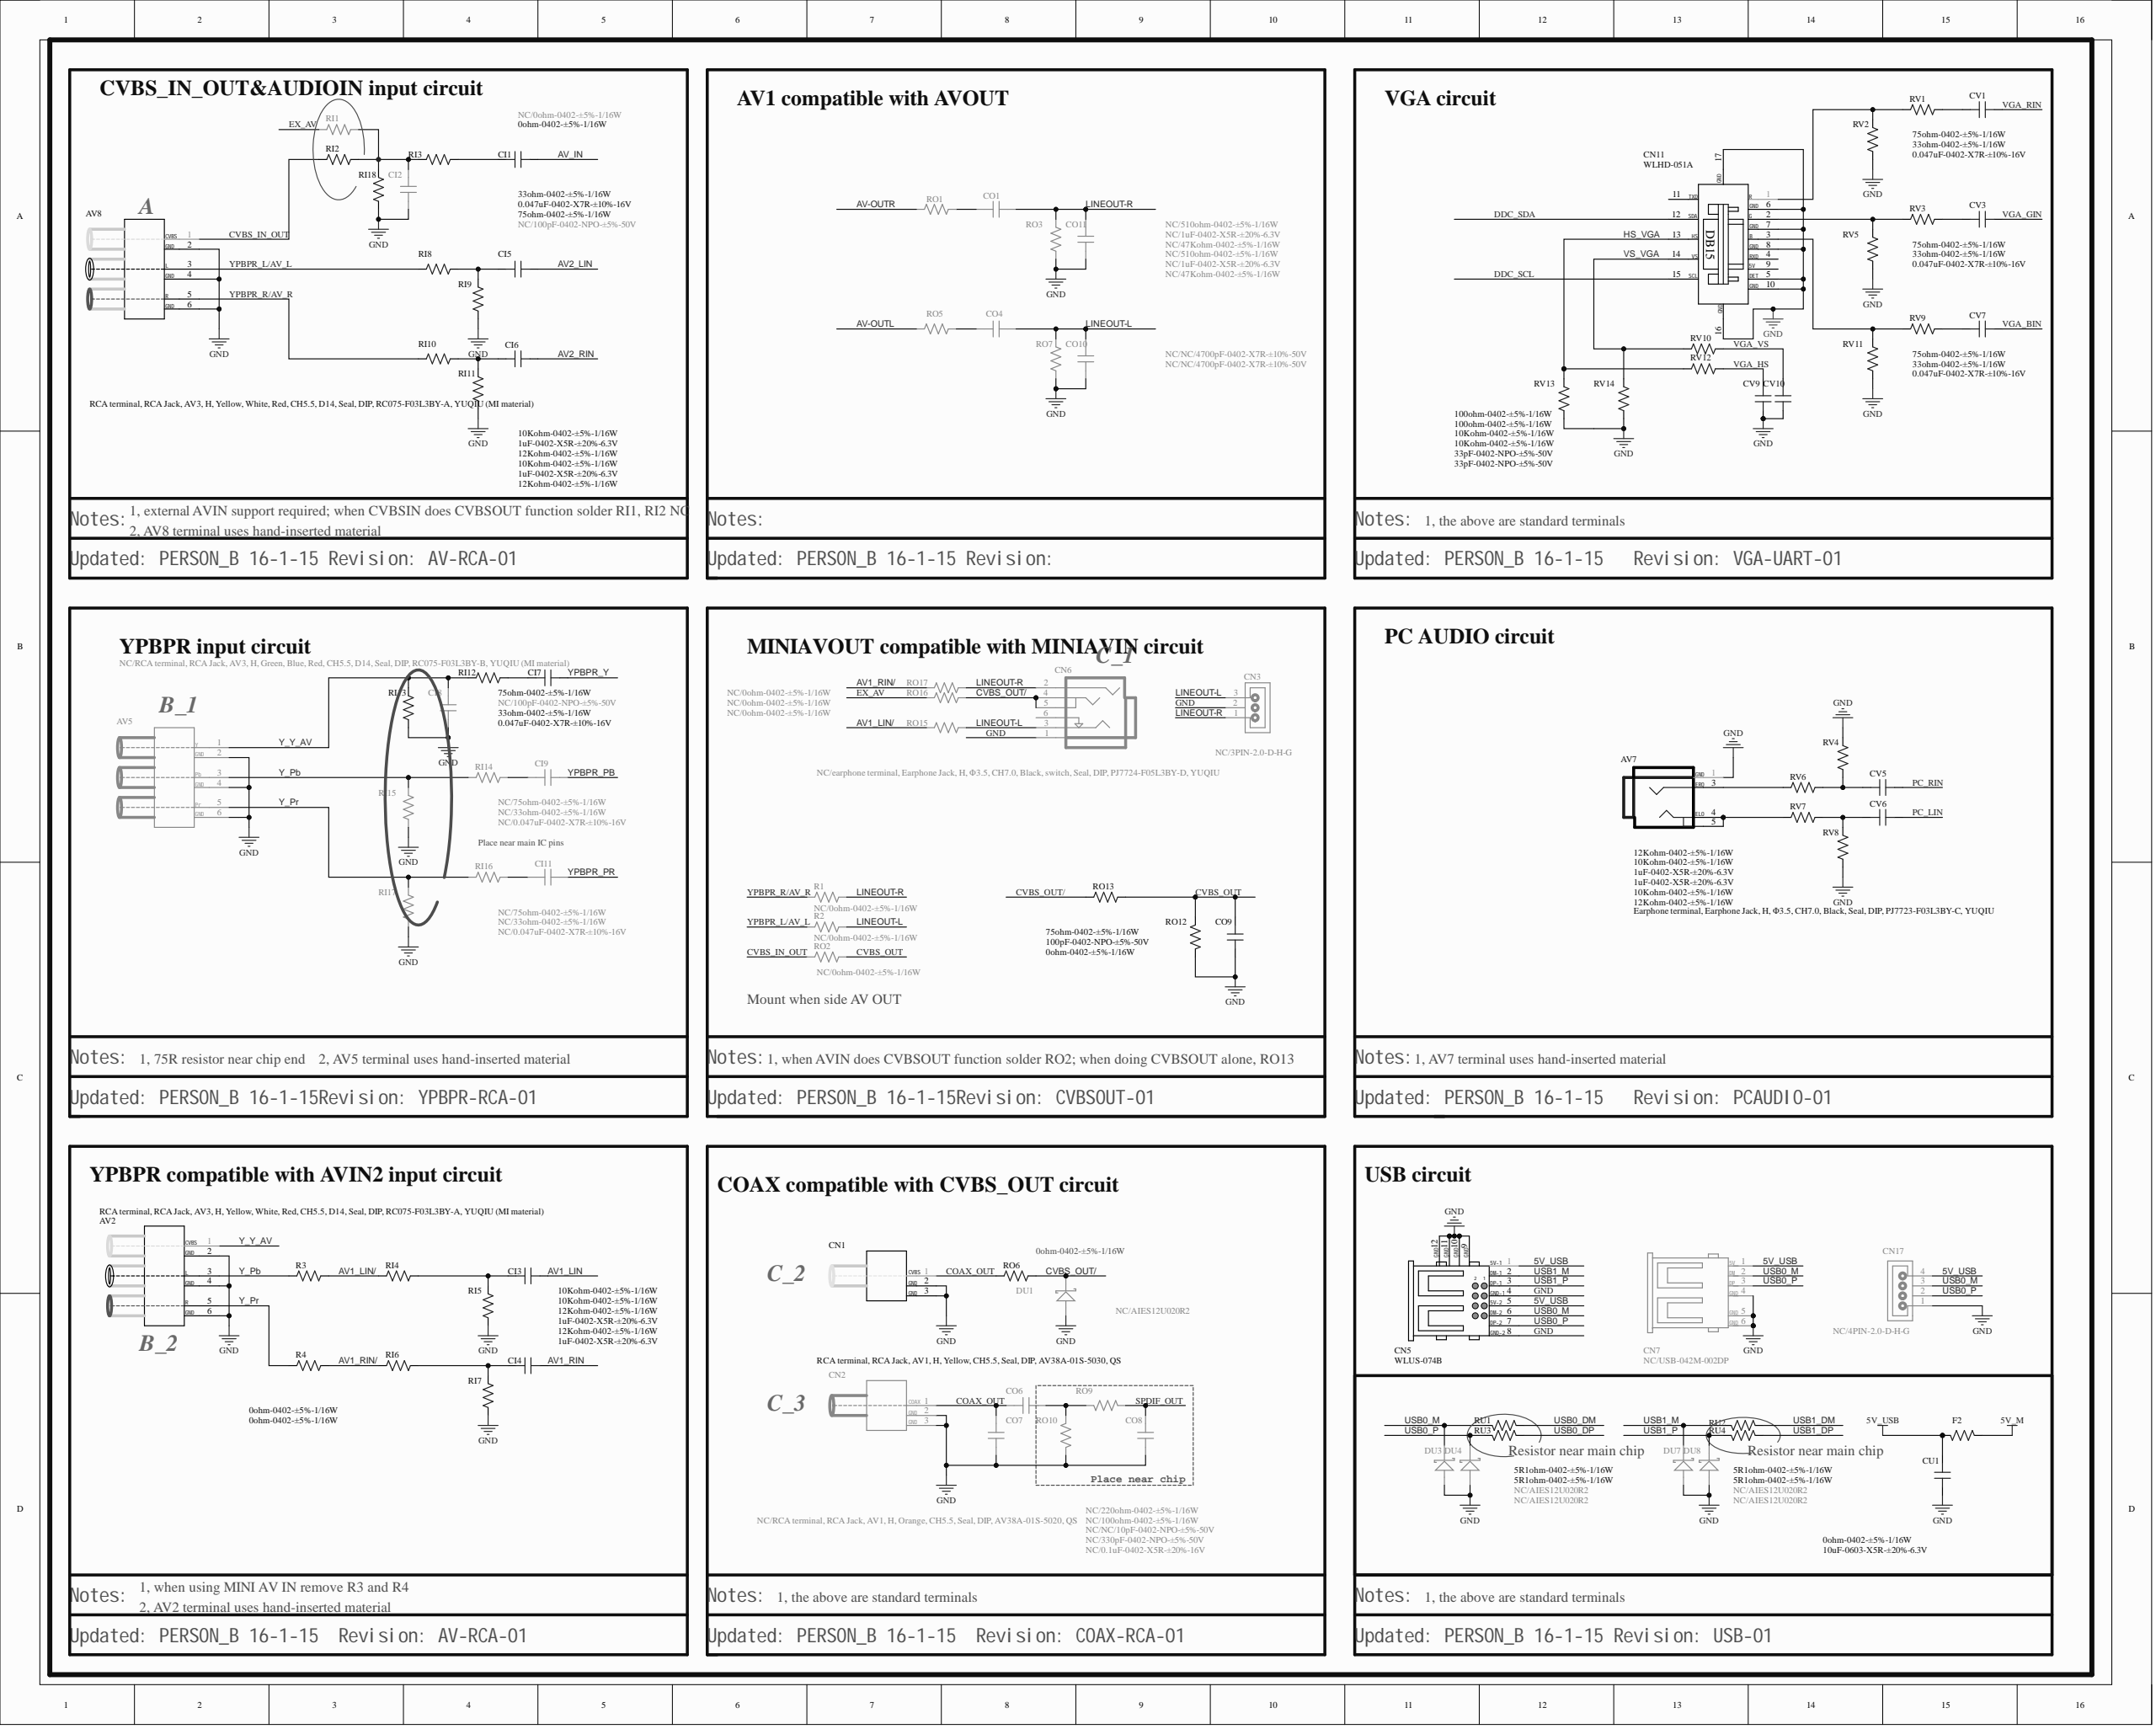Circuit board | Altium Designer | 709 parts | 378 nets | one sheet of the schematic
Parts on this sheet (reference | value | footprint):
AV2 | RCA terminal, RCA Jack, AV3, H, Yellow, White, Red, CH5.5, D14, Seal, DIP, RC075-F03L3BY-A, YUQIU (MI material) | AV3-H14-15
AV5 | NC/RCA terminal, RCA Jack, AV3, H, Green, Blue, Red, CH5.5, D14, Seal, DIP, RC075-F03L3BY-B, YUQIU (MI material) | AV3-H14-15
AV7 | Earphone terminal, Earphone Jack, H, F3.5, CH7.0, Black, Seal, DIP, PJ7723-F03L3BY-C, YUQIU | PHONE-HD-41
AV8 | RCA terminal, RCA Jack, AV3, H, Yellow, White, Red, CH5.5, D14, Seal, DIP, RC075-F03L3BY-A, YUQIU (MI material) | AV3-H14-15
CI1 | 0.047uF-0402-X7R-±10%-16V | C0402
CI2 | NC/100pF-0402-NPO-±5%-50V | C0402
CI3 | 1uF-0402-X5R-±20%-6.3V | C0402
CI4 | 1uF-0402-X5R-±20%-6.3V | C0402
CI5 | 1uF-0402-X5R-±20%-6.3V | C0402
CI6 | 1uF-0402-X5R-±20%-6.3V | C0402
CI7 | 0.047uF-0402-X7R-±10%-16V | C0402
CI8 | NC/100pF-0402-NPO-±5%-50V | C0402
CI9 | NC/0.047uF-0402-X7R-±10%-16V | C0402
CI11 | NC/0.047uF-0402-X7R-±10%-16V | C0402
CN1 | RCA terminal, RCA Jack, AV1, H, Yellow, CH5.5, Seal, DIP, AV38A-01S-5030, QS | AV1-H-4
CN2 | NC/RCA terminal, RCA Jack, AV1, H, Orange, CH5.5, Seal, DIP, AV38A-01S-5020, QS | AV1-H-4
CN3 | NC/3PIN-2.0-D-H-G | SIP3/2.0D-1
CN5 | WLUS-074B | USB2-HD-1
CN6 | NC/earphone terminal, Earphone Jack, H, F3.5, CH7.0, Black, switch, Seal, DIP, PJ7724-F05L3BY-D, YUQIU | PHONE-HD-42
CN7 | NC/USB-042M-002DP | USB1-HD-2
CN11 | WLHD-051A | DB15-HF-1
CN17 | NC/4PIN-2.0-D-H-G | SIP4/2.0D-1
CO1 | NC/1uF-0402-X5R-±20%-6.3V | C0402
CO4 | NC/1uF-0402-X5R-±20%-6.3V | C0402
CO6 | NC/0.1uF-0402-X5R-±20%-16V | C0402
CO7 | NC/330pF-0402-NPO-±5%-50V | C0402
CO8 | NC/NC/10pF-0402-NPO-±5%-50V | C0402
CO9 | 100pF-0402-NPO-±5%-50V | C0402
CO10 | NC/NC/4700pF-0402-X7R-±10%-50V | C0402
CO11 | NC/NC/4700pF-0402-X7R-±10%-50V | C0402
CU1 | 10uF-0603-X5R-±20%-6.3V | C0603
CV1 | 0.047uF-0402-X7R-±10%-16V | C0402
CV3 | 0.047uF-0402-X7R-±10%-16V | C0402
CV5 | 1uF-0402-X5R-±20%-6.3V | C0402
CV6 | 1uF-0402-X5R-±20%-6.3V | C0402
CV7 | 0.047uF-0402-X7R-±10%-16V | C0402
CV9 | 33pF-0402-NPO-±5%-50V | C0402
CV10 | 33pF-0402-NPO-±5%-50V | C0402
DU1 | NC/AIES12U020R2 | DIODE-S0402
DU3 | NC/AIES12U020R2 | DIODE-S0402
DU4 | NC/AIES12U020R2 | DIODE-S0402
DU7 | NC/AIES12U020R2 | DIODE-S0402
DU8 | NC/AIES12U020R2 | DIODE-S0402
F2 | 0ohm-0402-±5%-1/16W | R0402
R1 | NC/0ohm-0402-±5%-1/16W | R0402
R2 | NC/0ohm-0402-±5%-1/16W | R0402
R3 | 0ohm-0402-±5%-1/16W | R0402
R4 | 0ohm-0402-±5%-1/16W | R0402
RI1 | NC/0ohm-0402-±5%-1/16W | R0402
RI2 | 0ohm-0402-±5%-1/16W | R0402
RI3 | 33ohm-0402-±5%-1/16W | R0402
RI4 | 10Kohm-0402-±5%-1/16W | R0402
RI5 | 12Kohm-0402-±5%-1/16W | R0402
RI6 | 10Kohm-0402-±5%-1/16W | R0402
RI7 | 12Kohm-0402-±5%-1/16W | R0402
RI8 | 10Kohm-0402-±5%-1/16W | R0402
RI9 | 12Kohm-0402-±5%-1/16W | R0402
RI10 | 10Kohm-0402-±5%-1/16W | R0402
RI11 | 12Kohm-0402-±5%-1/16W | R0402
RI12 | 33ohm-0402-±5%-1/16W | R0402
RI13 | 75ohm-0402-±5%-1/16W | R0402
RI14 | NC/33ohm-0402-±5%-1/16W | R0402
RI15 | NC/75ohm-0402-±5%-1/16W | R0402
RI16 | NC/33ohm-0402-±5%-1/16W | R0402
RI17 | NC/75ohm-0402-±5%-1/16W | R0402
RI18 | 75ohm-0402-±5%-1/16W | R0402
RO1 | NC/510ohm-0402-±5%-1/16W | R0402
RO2 | NC/0ohm-0402-±5%-1/16W | R0402
RO3 | NC/47Kohm-0402-±5%-1/16W | R0402
RO5 | NC/510ohm-0402-±5%-1/16W | R0402
RO6 | 0ohm-0402-±5%-1/16W | R0402
RO7 | NC/47Kohm-0402-±5%-1/16W | R0402
RO9 | NC/220ohm-0402-±5%-1/16W | R0402
RO10 | NC/100ohm-0402-±5%-1/16W | R0402
RO12 | 75ohm-0402-±5%-1/16W | R0402
RO13 | 0ohm-0402-±5%-1/16W | R0402
RO15 | NC/0ohm-0402-±5%-1/16W | R0402
RO16 | NC/0ohm-0402-±5%-1/16W | R0402
RO17 | NC/0ohm-0402-±5%-1/16W | R0402
RU1 | 5R1ohm-0402-±5%-1/16W | R0402
RU2 | 5R1ohm-0402-±5%-1/16W | R0402
RU3 | 5R1ohm-0402-±5%-1/16W | R0402
RU4 | 5R1ohm-0402-±5%-1/16W | R0402
RV1 | 33ohm-0402-±5%-1/16W | R0402
RV2 | 75ohm-0402-±5%-1/16W | R0402
RV3 | 33ohm-0402-±5%-1/16W | R0402
RV4 | 12Kohm-0402-±5%-1/16W | R0402
RV5 | 75ohm-0402-±5%-1/16W | R0402
RV6 | 10Kohm-0402-±5%-1/16W | R0402
RV7 | 10Kohm-0402-±5%-1/16W | R0402
RV8 | 12Kohm-0402-±5%-1/16W | R0402
RV9 | 33ohm-0402-±5%-1/16W | R0402
RV10 | 100ohm-0402-±5%-1/16W | R0402
RV11 | 75ohm-0402-±5%-1/16W | R0402
RV12 | 100ohm-0402-±5%-1/16W | R0402
RV13 | 10Kohm-0402-±5%-1/16W | R0402
RV14 | 10Kohm-0402-±5%-1/16W | R0402
Nets of these parts (net: part-pin ...):
YPBPR_Y: CI7-1
YPBPR_R/AV_R: AV8-5 R1-1 RI10-2
YPBPR_PR: CI11-1
YPBPR_PB: CI9-1
YPBPR_L/AV_L: AV8-3 R2-1 RI8-2
Y_Y_AV: AV2-1 AV5-1 CI8-1 RI12-1 RI13-2
Y_Pr: AV2-5 AV5-5 R4-1 RI16-2 RI17-2
Y_Pb: AV2-3 AV5-3 R3-1 RI14-2 RI15-2
VS_VGA: CN11-14 RV10-1 RV14-1
VGA_VS: CV10-1 RV10-2
VGA_RIN: CV1-1
VGA_HS: CV9-1 RV12-2
VGA_GIN: CV3-1
VGA_BIN: CV7-1
USB1_P: CN5-3 DU8-K RU4-2
USB1_M: CN5-2 DU7-K RU2-2
USB1_DP: RU4-1
USB1_DM: RU2-1
USB0_P: CN5-7 CN7-3 CN17-2 DU4-K RU3-2
USB0_M: CN5-6 CN7-2 CN17-3 DU3-K RU1-2
USB0_DP: RU3-1
USB0_DM: RU1-1
SPDIF_OUT: CO8-1 RO9-1
PC_RIN: CV5-2
PC_LIN: CV6-2
NetCV7_2: CV7-2 RV9-1
NetCV6_1: CV6-1 RV7-1 RV8-1
NetCV5_1: CV5-1 RV4-2 RV6-1
NetCV3_2: CV3-2 RV3-1
NetCV1_2: CV1-2 RV1-1
NetCO6_2: CO6-2 RO9-2 RO10-1
NetCO4_2: CO4-2 RO5-2
NetCO1_2: CO1-2 RO1-2
NetCN11_3: CN11-3 RV9-2 RV11-2
NetCN11_2: CN11-2 RV3-2 RV5-2
NetCN11_1: CN11-1 RV1-2 RV2-2
NetCI11_2: CI11-2 RI16-1
NetCI9_2: CI9-2 RI14-1
NetCI7_2: CI7-2 RI12-2
NetCI6_2: CI6-2 RI10-1 RI11-1
NetCI5_2: CI5-2 RI8-1 RI9-2
NetCI4_2: CI4-2 RI6-1 RI7-1
NetCI3_2: CI3-2 RI4-1 RI5-2
NetCI2_1: CI2-1 RI1-2 RI2-2 RI3-2 RI18-2
NetCI1_2: CI1-2 RI3-1
NetAV7_4: AV7-4 AV7-5 RV7-2
NetAV7_3: AV7-3 RV6-2
LINEOUT-R: CN3-1 CN6-2 CO1-1 CO11-2 R1-2 RO3-2 RO17-2
LINEOUT-L: CN3-3 CN6-3 CO4-1 CO10-2 R2-2 RO7-2 RO15-2
HS_VGA: CN11-13 RV12-1 RV13-1
GND: AV2-2 AV2-4 AV2-6 AV5-2 AV5-4 AV5-6 AV7-1 AV8-2 AV8-4 AV8-6 CI2-2 CI8-2 CN1-2 CN1-3 CN2-2 CN2-3 CN3-2 CN5-4 CN5-8 CN5-9 CN5-10 CN5-11 CN5-12 CN6-1 CN7-4 CN7-5 CN7-6 CN11-5 CN11-6 CN11-7 CN11-8 CN11-10 CN11-16 CN11-17 CN17-1 CO7-2 CO8-2 CO9-1 CO10-1 CO11-1 CU1-1 CV9-2 CV10-2 DU1-A DU3-A DU4-A DU7-A DU8-A RI5-1 RI7-2 RI9-1 RI11-2 RI13-1 RI15-1 RI17-1 RI18-1 RO3-1 RO7-1 RO10-2 RO12-2 RV2-1 RV4-1 RV5-1 RV8-2 RV11-1 RV13-2 RV14-2
EX_AV: RI1-1 RO16-1
DDC_SDA: CN11-12
DDC_SCL: CN11-15
CVBS_OUT/: CN6-4 CN6-5 DU1-K RO6-2 RO13-1 RO16-2
CVBS_OUT: CO9-2 RO2-2 RO12-1 RO13-2
CVBS_IN_OUT: AV8-1 RI2-1 RO2-1
COAX_OUT: CN1-1 CN2-1 CO6-1 CO7-1 RO6-1
AV_IN: CI1-1
AV-OUTR: RO1-1
AV-OUTL: RO5-1
AV2_RIN: CI6-1
AV2_LIN: CI5-1
AV1_RIN/: R4-2 RI6-2 RO17-1
AV1_RIN: CI4-1
AV1_LIN/: R3-2 RI4-2 RO15-1
AV1_LIN: CI3-1
5V_USB: CN5-1 CN5-5 CN7-1 CN17-4 CU1-2 F2-2
5V_M: F2-1